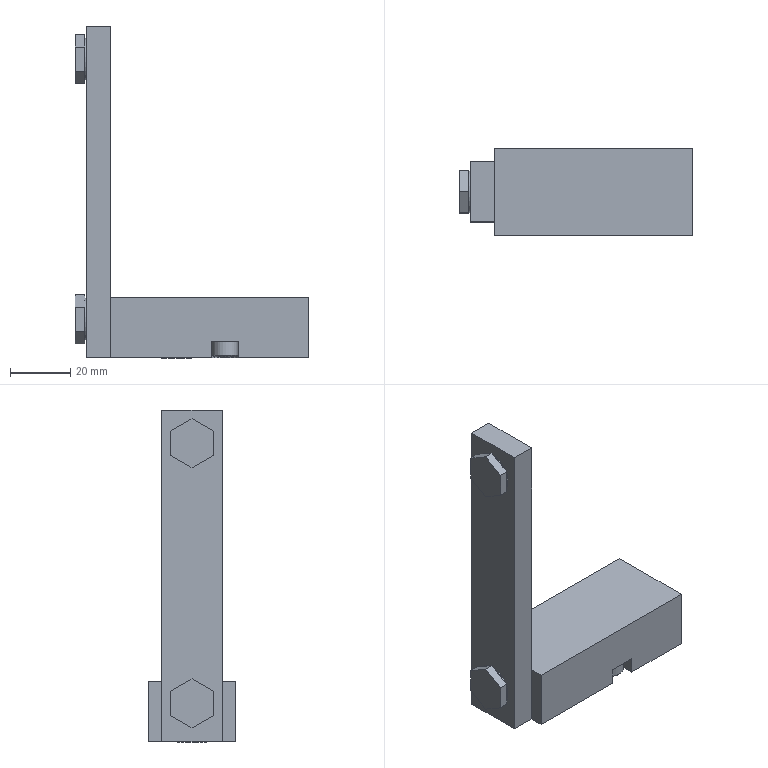Part | STEP file | _MXS20-50P(0)_FOP | 1 solid | 88 faces | box 77.2 x 29 x 110 mm | volume 55359 mm3 | plane 59 | cylinder 19 | cone 10 | commonest cylinder face diameters 8.5 x6 9 x5 8.566 x4 14 x4